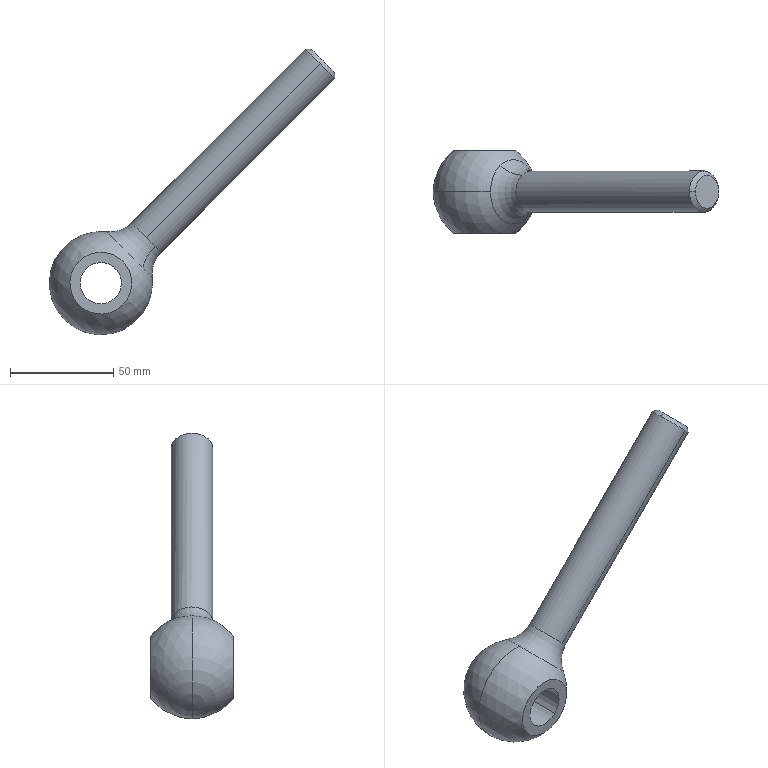Part | 1 solid | 13 faces | box 138.299 x 40 x 138.299 mm | volume 90064 mm3 | cylinder 4 | plane 3 | cone 2 | torus 2 | sphere 2 | commonest cylinder face diameters 20 x4
STEP:
#1=CARTESIAN_POINT('',(0.,0.,0.));
#2=DIRECTION('',(0.,0.,1.));
#3=DIRECTION('',(1.,0.,0.));
#4=AXIS2_PLACEMENT_3D('',#1,#2,#3);
#5=CARTESIAN_POINT('',(97.888,511.5,-299.372));
#6=VERTEX_POINT('',#5);
#7=CARTESIAN_POINT('',(13.739,511.5,-383.521));
#8=VERTEX_POINT('',#7);
#9=CARTESIAN_POINT('',(97.888,511.5,-299.372));
#10=DIRECTION('',(-0.7071,0.,-0.7071));
#11=VECTOR('',#10,1.);
#12=LINE('',#9,#11);
#13=CARTESIAN_POINT('',(-68.056,501.5,-465.316));
#14=DIRECTION('',(-0.7071,0.,-0.7071));
#15=DIRECTION('',(-0.7071,0.,0.7071));
#16=AXIS2_PLACEMENT_3D('',#13,#14,#15);
#17=CYLINDRICAL_SURFACE('',#16,10.);
#18=CARTESIAN_POINT('',(1.571,-234.68));
#19=DIRECTION('',(0.,1.));
#20=VECTOR('',#19,1.);
#21=LINE('',#18,#20);
#22=(GEOMETRIC_REPRESENTATION_CONTEXT(2)PARAMETRIC_REPRESENTATION_CONTEXT()REPRESENTATION_CONTEXT('',''));
#23=DEFINITIONAL_REPRESENTATION('',(#21),#22);
#24=PCURVE('',#17,#23);
#25=CARTESIAN_POINT('',(-68.056,501.5,-465.316));
#26=DIRECTION('',(-0.7071,0.,-0.7071));
#27=DIRECTION('',(0.7071,0.,-0.7071));
#28=AXIS2_PLACEMENT_3D('',#25,#26,#27);
#29=CYLINDRICAL_SURFACE('',#28,10.);
#30=CARTESIAN_POINT('',(4.712,-234.68));
#31=DIRECTION('',(0.,1.));
#32=VECTOR('',#31,1.);
#33=LINE('',#30,#32);
#34=(GEOMETRIC_REPRESENTATION_CONTEXT(2)PARAMETRIC_REPRESENTATION_CONTEXT()REPRESENTATION_CONTEXT('',''));
#35=DEFINITIONAL_REPRESENTATION('',(#33),#34);
#36=PCURVE('',#29,#35);
#37=SURFACE_CURVE('',#12,(#24,#36),.PCURVE_S1.);
#38=EDGE_CURVE('',#6,#8,#37,.T.);
#39=ORIENTED_EDGE('',*,*,#38,.F.);
#40=CARTESIAN_POINT('',(104.959,501.5,-306.443));
#41=VERTEX_POINT('',#40);
#42=CARTESIAN_POINT('',(97.888,501.5,-299.372));
#43=DIRECTION('',(-0.7071,0.,-0.7071));
#44=DIRECTION('',(0.7071,0.,-0.7071));
#45=AXIS2_PLACEMENT_3D('',#42,#43,#44);
#46=CIRCLE('',#45,10.);
#47=CARTESIAN_POINT('',(-3.142,-234.68));
#48=DIRECTION('',(1.,0.));
#49=VECTOR('',#48,1.);
#50=LINE('',#47,#49);
#51=(GEOMETRIC_REPRESENTATION_CONTEXT(2)PARAMETRIC_REPRESENTATION_CONTEXT()REPRESENTATION_CONTEXT('',''));
#52=DEFINITIONAL_REPRESENTATION('',(#50),#51);
#53=PCURVE('',#17,#52);
#54=CARTESIAN_POINT('',(97.888,501.5,-299.372));
#55=DIRECTION('',(-0.7071,0.,-0.7071));
#56=DIRECTION('',(0.,-1.,0.));
#57=AXIS2_PLACEMENT_3D('',#54,#55,#56);
#58=CONICAL_SURFACE('',#57,10.,0.7854);
#59=CARTESIAN_POINT('',(-1.571,0.));
#60=DIRECTION('',(1.,0.));
#61=VECTOR('',#60,1.);
#62=LINE('',#59,#61);
#63=(GEOMETRIC_REPRESENTATION_CONTEXT(2)PARAMETRIC_REPRESENTATION_CONTEXT()REPRESENTATION_CONTEXT('',''));
#64=DEFINITIONAL_REPRESENTATION('',(#62),#63);
#65=PCURVE('',#58,#64);
#66=SURFACE_CURVE('',#46,(#53,#65),.PCURVE_S1.);
#67=EDGE_CURVE('',#6,#41,#66,.T.);
#68=ORIENTED_EDGE('',*,*,#67,.T.);
#69=CARTESIAN_POINT('',(97.888,491.5,-299.372));
#70=VERTEX_POINT('',#69);
#71=CARTESIAN_POINT('',(97.888,501.5,-299.372));
#72=DIRECTION('',(-0.7071,0.,-0.7071));
#73=DIRECTION('',(0.7071,0.,-0.7071));
#74=AXIS2_PLACEMENT_3D('',#71,#72,#73);
#75=CIRCLE('',#74,10.);
#76=CARTESIAN_POINT('',(3.142,-234.68));
#77=DIRECTION('',(1.,0.));
#78=VECTOR('',#77,1.);
#79=LINE('',#76,#78);
#80=(GEOMETRIC_REPRESENTATION_CONTEXT(2)PARAMETRIC_REPRESENTATION_CONTEXT()REPRESENTATION_CONTEXT('',''));
#81=DEFINITIONAL_REPRESENTATION('',(#79),#80);
#82=PCURVE('',#17,#81);
#83=CARTESIAN_POINT('',(97.888,501.5,-299.372));
#84=DIRECTION('',(-0.7071,0.,-0.7071));
#85=DIRECTION('',(0.,1.,0.));
#86=AXIS2_PLACEMENT_3D('',#83,#84,#85);
#87=CONICAL_SURFACE('',#86,10.,0.7854);
#88=CARTESIAN_POINT('',(1.571,0.));
#89=DIRECTION('',(1.,0.));
#90=VECTOR('',#89,1.);
#91=LINE('',#88,#90);
#92=(GEOMETRIC_REPRESENTATION_CONTEXT(2)PARAMETRIC_REPRESENTATION_CONTEXT()REPRESENTATION_CONTEXT('',''));
#93=DEFINITIONAL_REPRESENTATION('',(#91),#92);
#94=PCURVE('',#87,#93);
#95=SURFACE_CURVE('',#75,(#82,#94),.PCURVE_S1.);
#96=EDGE_CURVE('',#41,#70,#95,.T.);
#97=ORIENTED_EDGE('',*,*,#96,.T.);
#98=CARTESIAN_POINT('',(13.739,491.5,-383.521));
#99=VERTEX_POINT('',#98);
#100=CARTESIAN_POINT('',(97.888,491.5,-299.372));
#101=DIRECTION('',(-0.7071,0.,-0.7071));
#102=VECTOR('',#101,1.);
#103=LINE('',#100,#102);
#104=CARTESIAN_POINT('',(4.712,-234.68));
#105=DIRECTION('',(0.,1.));
#106=VECTOR('',#105,1.);
#107=LINE('',#104,#106);
#108=(GEOMETRIC_REPRESENTATION_CONTEXT(2)PARAMETRIC_REPRESENTATION_CONTEXT()REPRESENTATION_CONTEXT('',''));
#109=DEFINITIONAL_REPRESENTATION('',(#107),#108);
#110=PCURVE('',#17,#109);
#111=CARTESIAN_POINT('',(1.571,-234.68));
#112=DIRECTION('',(0.,1.));
#113=VECTOR('',#112,1.);
#114=LINE('',#111,#113);
#115=(GEOMETRIC_REPRESENTATION_CONTEXT(2)PARAMETRIC_REPRESENTATION_CONTEXT()REPRESENTATION_CONTEXT('',''));
#116=DEFINITIONAL_REPRESENTATION('',(#114),#115);
#117=PCURVE('',#29,#116);
#118=SURFACE_CURVE('',#103,(#110,#117),.PCURVE_S1.);
#119=EDGE_CURVE('',#70,#99,#118,.T.);
#120=ORIENTED_EDGE('',*,*,#119,.T.);
#121=CARTESIAN_POINT('',(17.896,493.41,-387.677));
#122=VERTEX_POINT('',#121);
#123=CARTESIAN_POINT('',(13.739,501.5,-383.521));
#124=DIRECTION('',(-0.7071,0.,-0.7071));
#125=DIRECTION('',(0.,-1.,0.));
#126=AXIS2_PLACEMENT_3D('',#123,#124,#125);
#127=CIRCLE('',#126,10.);
#128=CARTESIAN_POINT('',(-1.571,-115.676));
#129=DIRECTION('',(1.,0.));
#130=VECTOR('',#129,1.);
#131=LINE('',#128,#130);
#132=(GEOMETRIC_REPRESENTATION_CONTEXT(2)PARAMETRIC_REPRESENTATION_CONTEXT()REPRESENTATION_CONTEXT('',''));
#133=DEFINITIONAL_REPRESENTATION('',(#131),#132);
#134=PCURVE('',#17,#133);
#135=CARTESIAN_POINT('',(13.739,501.5,-383.521));
#136=DIRECTION('',(-0.7071,0.,-0.7071));
#137=DIRECTION('',(0.5721,0.5878,-0.5721));
#138=AXIS2_PLACEMENT_3D('',#135,#136,#137);
#139=TOROIDAL_SURFACE('',#138,25.,15.);
#140=CARTESIAN_POINT('',(-4.084,3.142));
#141=DIRECTION('',(1.,0.));
#142=VECTOR('',#141,1.);
#143=LINE('',#140,#142);
#144=(GEOMETRIC_REPRESENTATION_CONTEXT(2)PARAMETRIC_REPRESENTATION_CONTEXT()REPRESENTATION_CONTEXT('',''));
#145=DEFINITIONAL_REPRESENTATION('',(#143),#144);
#146=PCURVE('',#139,#145);
#147=SURFACE_CURVE('',#127,(#134,#146),.PCURVE_S1.);
#148=EDGE_CURVE('',#122,#99,#147,.T.);
#149=ORIENTED_EDGE('',*,*,#148,.F.);
#150=CARTESIAN_POINT('',(13.739,501.5,-383.521));
#151=DIRECTION('',(-0.7071,0.,-0.7071));
#152=DIRECTION('',(0.,-1.,0.));
#153=AXIS2_PLACEMENT_3D('',#150,#151,#152);
#154=CIRCLE('',#153,10.);
#155=CARTESIAN_POINT('',(-1.571,-115.676));
#156=DIRECTION('',(1.,0.));
#157=VECTOR('',#156,1.);
#158=LINE('',#155,#157);
#159=(GEOMETRIC_REPRESENTATION_CONTEXT(2)PARAMETRIC_REPRESENTATION_CONTEXT()REPRESENTATION_CONTEXT('',''));
#160=DEFINITIONAL_REPRESENTATION('',(#158),#159);
#161=PCURVE('',#17,#160);
#162=CARTESIAN_POINT('',(13.739,501.5,-383.521));
#163=DIRECTION('',(-0.7071,0.,-0.7071));
#164=DIRECTION('',(-0.5721,-0.5878,0.5721));
#165=AXIS2_PLACEMENT_3D('',#162,#163,#164);
#166=TOROIDAL_SURFACE('',#165,25.,15.);
#167=CARTESIAN_POINT('',(-0.9425,3.142));
#168=DIRECTION('',(1.,0.));
#169=VECTOR('',#168,1.);
#170=LINE('',#167,#169);
#171=(GEOMETRIC_REPRESENTATION_CONTEXT(2)PARAMETRIC_REPRESENTATION_CONTEXT()REPRESENTATION_CONTEXT('',''));
#172=DEFINITIONAL_REPRESENTATION('',(#170),#171);
#173=PCURVE('',#166,#172);
#174=SURFACE_CURVE('',#154,(#161,#173),.PCURVE_S1.);
#175=EDGE_CURVE('',#8,#122,#174,.T.);
#176=ORIENTED_EDGE('',*,*,#175,.F.);
#177=EDGE_LOOP('',(#39,#68,#97,#120,#149,#176));
#178=FACE_BOUND('',#177,.T.);
#179=ADVANCED_FACE('',(#178),#17,.T.);
#180=CARTESIAN_POINT('',(93.646,501.5,-292.301));
#181=VERTEX_POINT('',#180);
#182=CARTESIAN_POINT('',(90.817,501.5,-292.301));
#183=VERTEX_POINT('',#182);
#184=CARTESIAN_POINT('',(93.646,501.5,-292.301));
#185=DIRECTION('',(-1.,0.,-0.000000001));
#186=VECTOR('',#185,1.);
#187=LINE('',#184,#186);
#188=CARTESIAN_POINT('',(1.571,-2.));
#189=DIRECTION('',(0.,1.));
#190=VECTOR('',#189,1.);
#191=LINE('',#188,#190);
#192=(GEOMETRIC_REPRESENTATION_CONTEXT(2)PARAMETRIC_REPRESENTATION_CONTEXT()REPRESENTATION_CONTEXT('',''));
#193=DEFINITIONAL_REPRESENTATION('',(#191),#192);
#194=PCURVE('',#58,#193);
#195=CARTESIAN_POINT('',(4.712,-2.));
#196=DIRECTION('',(0.,1.));
#197=VECTOR('',#196,1.);
#198=LINE('',#195,#197);
#199=(GEOMETRIC_REPRESENTATION_CONTEXT(2)PARAMETRIC_REPRESENTATION_CONTEXT()REPRESENTATION_CONTEXT('',''));
#200=DEFINITIONAL_REPRESENTATION('',(#198),#199);
#201=PCURVE('',#87,#200);
#202=SURFACE_CURVE('',#187,(#194,#201),.PCURVE_S1.);
#203=EDGE_CURVE('',#181,#183,#202,.T.);
#204=ORIENTED_EDGE('',*,*,#203,.F.);
#205=CARTESIAN_POINT('',(104.959,501.5,-303.614));
#206=VERTEX_POINT('',#205);
#207=CARTESIAN_POINT('',(99.303,501.5,-297.958));
#208=DIRECTION('',(0.7071,0.,0.7071));
#209=DIRECTION('',(0.7071,0.,-0.7071));
#210=AXIS2_PLACEMENT_3D('',#207,#208,#209);
#211=CIRCLE('',#210,8.);
#212=CARTESIAN_POINT('',(4.712,-2.));
#213=DIRECTION('',(-1.,0.));
#214=VECTOR('',#213,1.);
#215=LINE('',#212,#214);
#216=(GEOMETRIC_REPRESENTATION_CONTEXT(2)PARAMETRIC_REPRESENTATION_CONTEXT()REPRESENTATION_CONTEXT('',''));
#217=DEFINITIONAL_REPRESENTATION('',(#215),#216);
#218=PCURVE('',#58,#217);
#219=CARTESIAN_POINT('',(93.646,501.5,-292.301));
#220=DIRECTION('',(0.7071,0.,0.7071));
#221=DIRECTION('',(0.,1.,0.));
#222=AXIS2_PLACEMENT_3D('',#219,#220,#221);
#223=PLANE('',#222);
#224=CARTESIAN_POINT('',(0.,-8.));
#225=DIRECTION('',(0.,-1.));
#226=AXIS2_PLACEMENT_2D('',#224,#225);
#227=CIRCLE('',#226,8.);
#228=(GEOMETRIC_REPRESENTATION_CONTEXT(2)PARAMETRIC_REPRESENTATION_CONTEXT()REPRESENTATION_CONTEXT('',''));
#229=DEFINITIONAL_REPRESENTATION('',(#227),#228);
#230=PCURVE('',#223,#229);
#231=SURFACE_CURVE('',#211,(#218,#230),.PCURVE_S1.);
#232=EDGE_CURVE('',#206,#181,#231,.T.);
#233=ORIENTED_EDGE('',*,*,#232,.F.);
#234=CARTESIAN_POINT('',(104.959,501.5,-303.614));
#235=DIRECTION('',(0.,0.,-1.));
#236=VECTOR('',#235,1.);
#237=LINE('',#234,#236);
#238=CARTESIAN_POINT('',(4.712,-2.));
#239=DIRECTION('',(0.,1.));
#240=VECTOR('',#239,1.);
#241=LINE('',#238,#240);
#242=(GEOMETRIC_REPRESENTATION_CONTEXT(2)PARAMETRIC_REPRESENTATION_CONTEXT()REPRESENTATION_CONTEXT('',''));
#243=DEFINITIONAL_REPRESENTATION('',(#241),#242);
#244=PCURVE('',#58,#243);
#245=CARTESIAN_POINT('',(1.571,-2.));
#246=DIRECTION('',(0.,1.));
#247=VECTOR('',#246,1.);
#248=LINE('',#245,#247);
#249=(GEOMETRIC_REPRESENTATION_CONTEXT(2)PARAMETRIC_REPRESENTATION_CONTEXT()REPRESENTATION_CONTEXT('',''));
#250=DEFINITIONAL_REPRESENTATION('',(#248),#249);
#251=PCURVE('',#87,#250);
#252=SURFACE_CURVE('',#237,(#244,#251),.PCURVE_S1.);
#253=EDGE_CURVE('',#206,#41,#252,.T.);
#254=ORIENTED_EDGE('',*,*,#253,.T.);
#255=ORIENTED_EDGE('',*,*,#67,.F.);
#256=CARTESIAN_POINT('',(97.888,501.5,-299.372));
#257=DIRECTION('',(-0.7071,0.,-0.7071));
#258=DIRECTION('',(0.7071,0.,-0.7071));
#259=AXIS2_PLACEMENT_3D('',#256,#257,#258);
#260=CIRCLE('',#259,10.);
#261=CARTESIAN_POINT('',(-1.571,0.));
#262=DIRECTION('',(1.,0.));
#263=VECTOR('',#262,1.);
#264=LINE('',#261,#263);
#265=(GEOMETRIC_REPRESENTATION_CONTEXT(2)PARAMETRIC_REPRESENTATION_CONTEXT()REPRESENTATION_CONTEXT('',''));
#266=DEFINITIONAL_REPRESENTATION('',(#264),#265);
#267=PCURVE('',#58,#266);
#268=CARTESIAN_POINT('',(0.,-234.68));
#269=DIRECTION('',(1.,0.));
#270=VECTOR('',#269,1.);
#271=LINE('',#268,#270);
#272=(GEOMETRIC_REPRESENTATION_CONTEXT(2)PARAMETRIC_REPRESENTATION_CONTEXT()REPRESENTATION_CONTEXT('',''));
#273=DEFINITIONAL_REPRESENTATION('',(#271),#272);
#274=PCURVE('',#29,#273);
#275=SURFACE_CURVE('',#260,(#267,#274),.PCURVE_S1.);
#276=EDGE_CURVE('',#183,#6,#275,.T.);
#277=ORIENTED_EDGE('',*,*,#276,.F.);
#278=EDGE_LOOP('',(#204,#233,#254,#255,#277));
#279=FACE_BOUND('',#278,.T.);
#280=ADVANCED_FACE('',(#279),#58,.T.);
#281=ORIENTED_EDGE('',*,*,#232,.T.);
#282=CARTESIAN_POINT('',(99.303,501.5,-297.958));
#283=DIRECTION('',(0.7071,0.,0.7071));
#284=DIRECTION('',(0.7071,0.,-0.7071));
#285=AXIS2_PLACEMENT_3D('',#282,#283,#284);
#286=CIRCLE('',#285,8.);
#287=CARTESIAN_POINT('',(0.,-8.));
#288=DIRECTION('',(0.,-1.));
#289=AXIS2_PLACEMENT_2D('',#287,#288);
#290=CIRCLE('',#289,8.);
#291=(GEOMETRIC_REPRESENTATION_CONTEXT(2)PARAMETRIC_REPRESENTATION_CONTEXT()REPRESENTATION_CONTEXT('',''));
#292=DEFINITIONAL_REPRESENTATION('',(#290),#291);
#293=PCURVE('',#223,#292);
#294=CARTESIAN_POINT('',(7.854,-2.));
#295=DIRECTION('',(-1.,0.));
#296=VECTOR('',#295,1.);
#297=LINE('',#294,#296);
#298=(GEOMETRIC_REPRESENTATION_CONTEXT(2)PARAMETRIC_REPRESENTATION_CONTEXT()REPRESENTATION_CONTEXT('',''));
#299=DEFINITIONAL_REPRESENTATION('',(#297),#298);
#300=PCURVE('',#87,#299);
#301=SURFACE_CURVE('',#286,(#293,#300),.PCURVE_S1.);
#302=EDGE_CURVE('',#181,#206,#301,.T.);
#303=ORIENTED_EDGE('',*,*,#302,.T.);
#304=EDGE_LOOP('',(#281,#303));
#305=FACE_BOUND('',#304,.T.);
#306=ADVANCED_FACE('',(#305),#223,.T.);
#307=CARTESIAN_POINT('',(-1.034,514.141,-385.306));
#308=VERTEX_POINT('',#307);
#309=CARTESIAN_POINT('',(16.508,501.5,-402.849));
#310=VERTEX_POINT('',#309);
#311=CARTESIAN_POINT('',(5.46,501.5,-391.8));
#312=DIRECTION('',(-0.7071,0.,-0.7071));
#313=DIRECTION('',(0.7071,0.,-0.7071));
#314=AXIS2_PLACEMENT_3D('',#311,#312,#313);
#315=CIRCLE('',#314,15.625);
#316=CARTESIAN_POINT('',(-2.513,2.246));
#317=DIRECTION('',(1.,0.));
#318=VECTOR('',#317,1.);
#319=LINE('',#316,#318);
#320=(GEOMETRIC_REPRESENTATION_CONTEXT(2)PARAMETRIC_REPRESENTATION_CONTEXT()REPRESENTATION_CONTEXT('',''));
#321=DEFINITIONAL_REPRESENTATION('',(#319),#320);
#322=PCURVE('',#166,#321);
#323=CARTESIAN_POINT('',(-8.34,501.5,-405.6));
#324=DIRECTION('',(-0.7071,0.,-0.7071));
#325=DIRECTION('',(0.,-1.,0.));
#326=AXIS2_PLACEMENT_3D('',#323,#324,#325);
#327=SPHERICAL_SURFACE('',#326,25.);
#328=CARTESIAN_POINT('',(-1.571,-0.8957));
#329=DIRECTION('',(1.,0.));
#330=VECTOR('',#329,1.);
#331=LINE('',#328,#330);
#332=(GEOMETRIC_REPRESENTATION_CONTEXT(2)PARAMETRIC_REPRESENTATION_CONTEXT()REPRESENTATION_CONTEXT('',''));
#333=DEFINITIONAL_REPRESENTATION('',(#331),#332);
#334=PCURVE('',#327,#333);
#335=SURFACE_CURVE('',#315,(#322,#334),.PCURVE_S1.);
#336=EDGE_CURVE('',#308,#310,#335,.T.);
#337=ORIENTED_EDGE('',*,*,#336,.T.);
#338=CARTESIAN_POINT('',(11.954,488.859,-398.295));
#339=VERTEX_POINT('',#338);
#340=CARTESIAN_POINT('',(5.46,501.5,-391.8));
#341=DIRECTION('',(-0.7071,0.,-0.7071));
#342=DIRECTION('',(0.7071,0.,-0.7071));
#343=AXIS2_PLACEMENT_3D('',#340,#341,#342);
#344=CIRCLE('',#343,15.625);
#345=CARTESIAN_POINT('',(3.77,2.246));
#346=DIRECTION('',(1.,0.));
#347=VECTOR('',#346,1.);
#348=LINE('',#345,#347);
#349=(GEOMETRIC_REPRESENTATION_CONTEXT(2)PARAMETRIC_REPRESENTATION_CONTEXT()REPRESENTATION_CONTEXT('',''));
#350=DEFINITIONAL_REPRESENTATION('',(#348),#349);
#351=PCURVE('',#166,#350);
#352=CARTESIAN_POINT('',(-8.34,501.5,-405.6));
#353=DIRECTION('',(-0.7071,0.,-0.7071));
#354=DIRECTION('',(0.,1.,0.));
#355=AXIS2_PLACEMENT_3D('',#352,#353,#354);
#356=SPHERICAL_SURFACE('',#355,25.);
#357=CARTESIAN_POINT('',(1.571,-0.8957));
#358=DIRECTION('',(1.,0.));
#359=VECTOR('',#358,1.);
#360=LINE('',#357,#359);
#361=(GEOMETRIC_REPRESENTATION_CONTEXT(2)PARAMETRIC_REPRESENTATION_CONTEXT()REPRESENTATION_CONTEXT('',''));
#362=DEFINITIONAL_REPRESENTATION('',(#360),#361);
#363=PCURVE('',#356,#362);
#364=SURFACE_CURVE('',#344,(#351,#363),.PCURVE_S1.);
#365=EDGE_CURVE('',#310,#339,#364,.T.);
#366=ORIENTED_EDGE('',*,*,#365,.T.);
#367=CARTESIAN_POINT('',(24.13,481.275,-393.911));
#368=DIRECTION('',(-0.5721,-0.5878,0.5721));
#369=DIRECTION('',(-0.4156,0.809,0.4156));
#370=AXIS2_PLACEMENT_3D('',#367,#368,#369);
#371=CIRCLE('',#370,15.);
#372=CARTESIAN_POINT('',(4.712,3.142));
#373=DIRECTION('',(0.,-1.));
#374=VECTOR('',#373,1.);
#375=LINE('',#372,#374);
#376=(GEOMETRIC_REPRESENTATION_CONTEXT(2)PARAMETRIC_REPRESENTATION_CONTEXT()REPRESENTATION_CONTEXT('',''));
#377=DEFINITIONAL_REPRESENTATION('',(#375),#376);
#378=PCURVE('',#166,#377);
#379=CARTESIAN_POINT('',(1.571,3.142));
#380=DIRECTION('',(0.,-1.));
#381=VECTOR('',#380,1.);
#382=LINE('',#379,#381);
#383=(GEOMETRIC_REPRESENTATION_CONTEXT(2)PARAMETRIC_REPRESENTATION_CONTEXT()REPRESENTATION_CONTEXT('',''));
#384=DEFINITIONAL_REPRESENTATION('',(#382),#383);
#385=PCURVE('',#139,#384);
#386=SURFACE_CURVE('',#371,(#378,#385),.PCURVE_S1.);
#387=EDGE_CURVE('',#122,#339,#386,.T.);
#388=ORIENTED_EDGE('',*,*,#387,.F.);
#389=ORIENTED_EDGE('',*,*,#175,.F.);
#390=CARTESIAN_POINT('',(9.583,509.59,-379.364));
#391=VERTEX_POINT('',#390);
#392=CARTESIAN_POINT('',(13.739,501.5,-383.521));
#393=DIRECTION('',(-0.7071,0.,-0.7071));
#394=DIRECTION('',(0.,-1.,0.));
#395=AXIS2_PLACEMENT_3D('',#392,#393,#394);
#396=CIRCLE('',#395,10.);
#397=CARTESIAN_POINT('',(-0.9425,3.142));
#398=DIRECTION('',(1.,0.));
#399=VECTOR('',#398,1.);
#400=LINE('',#397,#399);
#401=(GEOMETRIC_REPRESENTATION_CONTEXT(2)PARAMETRIC_REPRESENTATION_CONTEXT()REPRESENTATION_CONTEXT('',''));
#402=DEFINITIONAL_REPRESENTATION('',(#400),#401);
#403=PCURVE('',#166,#402);
#404=CARTESIAN_POINT('',(1.571,-115.676));
#405=DIRECTION('',(1.,0.));
#406=VECTOR('',#405,1.);
#407=LINE('',#404,#406);
#408=(GEOMETRIC_REPRESENTATION_CONTEXT(2)PARAMETRIC_REPRESENTATION_CONTEXT()REPRESENTATION_CONTEXT('',''));
#409=DEFINITIONAL_REPRESENTATION('',(#407),#408);
#410=PCURVE('',#29,#409);
#411=SURFACE_CURVE('',#396,(#403,#410),.PCURVE_S1.);
#412=EDGE_CURVE('',#391,#8,#411,.T.);
#413=ORIENTED_EDGE('',*,*,#412,.F.);
#414=CARTESIAN_POINT('',(3.349,521.725,-373.13));
#415=DIRECTION('',(0.5721,0.5878,-0.5721));
#416=DIRECTION('',(0.4156,-0.809,-0.4156));
#417=AXIS2_PLACEMENT_3D('',#414,#415,#416);
#418=CIRCLE('',#417,15.);
#419=CARTESIAN_POINT('',(1.571,3.142));
#420=DIRECTION('',(0.,-1.));
#421=VECTOR('',#420,1.);
#422=LINE('',#419,#421);
#423=(GEOMETRIC_REPRESENTATION_CONTEXT(2)PARAMETRIC_REPRESENTATION_CONTEXT()REPRESENTATION_CONTEXT('',''));
#424=DEFINITIONAL_REPRESENTATION('',(#422),#423);
#425=PCURVE('',#166,#424);
#426=CARTESIAN_POINT('',(4.712,3.142));
#427=DIRECTION('',(0.,-1.));
#428=VECTOR('',#427,1.);
#429=LINE('',#426,#428);
#430=(GEOMETRIC_REPRESENTATION_CONTEXT(2)PARAMETRIC_REPRESENTATION_CONTEXT()REPRESENTATION_CONTEXT('',''));
#431=DEFINITIONAL_REPRESENTATION('',(#429),#430);
#432=PCURVE('',#139,#431);
#433=SURFACE_CURVE('',#418,(#425,#432),.PCURVE_S1.);
#434=EDGE_CURVE('',#391,#308,#433,.T.);
#435=ORIENTED_EDGE('',*,*,#434,.T.);
#436=EDGE_LOOP('',(#337,#366,#388,#389,#413,#435));
#437=FACE_BOUND('',#436,.F.);
#438=ADVANCED_FACE('',(#437),#166,.F.);
#439=CARTESIAN_POINT('',(-26.018,501.5,-423.278));
#440=VERTEX_POINT('',#439);
#441=CARTESIAN_POINT('',(-5.589,501.5,-380.752));
#442=VERTEX_POINT('',#441);
#443=CARTESIAN_POINT('',(-8.34,501.5,-405.6));
#444=DIRECTION('',(0.,1.,0.));
#445=DIRECTION('',(-0.7071,0.,-0.7071));
#446=AXIS2_PLACEMENT_3D('',#443,#444,#445);
#447=CIRCLE('',#446,25.);
#448=CARTESIAN_POINT('',(1.571,1.571));
#449=CARTESIAN_POINT('',(1.571,1.533));
#450=CARTESIAN_POINT('',(1.571,1.459));
#451=CARTESIAN_POINT('',(1.571,1.347));
#452=CARTESIAN_POINT('',(1.571,1.234));
#453=CARTESIAN_POINT('',(1.571,1.122));
#454=CARTESIAN_POINT('',(1.571,1.01));
#455=CARTESIAN_POINT('',(1.571,0.8981));
#456=CARTESIAN_POINT('',(1.571,0.786));
#457=CARTESIAN_POINT('',(1.571,0.6739));
#458=CARTESIAN_POINT('',(1.571,0.5618));
#459=CARTESIAN_POINT('',(1.571,0.4497));
#460=CARTESIAN_POINT('',(1.571,0.3376));
#461=CARTESIAN_POINT('',(1.571,0.2255));
#462=CARTESIAN_POINT('',(1.571,0.1133));
#463=CARTESIAN_POINT('',(1.571,0.00123));
#464=CARTESIAN_POINT('',(1.571,-0.1109));
#465=CARTESIAN_POINT('',(1.571,-0.223));
#466=CARTESIAN_POINT('',(1.571,-0.3351));
#467=CARTESIAN_POINT('',(1.571,-0.4472));
#468=CARTESIAN_POINT('',(1.571,-0.5593));
#469=CARTESIAN_POINT('',(1.571,-0.6714));
#470=CARTESIAN_POINT('',(1.571,-0.7836));
#471=CARTESIAN_POINT('',(1.571,-0.8583));
#472=CARTESIAN_POINT('',(1.571,-0.8957));
#473=B_SPLINE_CURVE_WITH_KNOTS('',3,(#448,#449,#450,#451,#452,#453,#454,#455,#456,#457,#458,#459,#460,#461,#462,#463,#464,#465,#466,#467,#468,#469,#470,#471,#472),.UNSPECIFIED.,.F.,.F.,(4,1,1,1,1,1,1,1,1,1,1,1,1,1,1,1,1,1,1,1,1,1,4),(0.,0.1121,0.2242,0.3363,0.4484,0.5606,0.6727,0.7848,0.8969,1.009,1.121,1.233,1.345,1.457,1.57,1.682,1.794,1.906,2.018,2.13,2.242,2.354,2.466),.QUASI_UNIFORM_KNOTS.);
#474=(GEOMETRIC_REPRESENTATION_CONTEXT(2)PARAMETRIC_REPRESENTATION_CONTEXT()REPRESENTATION_CONTEXT('',''));
#475=DEFINITIONAL_REPRESENTATION('',(#473),#474);
#476=PCURVE('',#327,#475);
#477=CARTESIAN_POINT('',(4.712,1.571));
#478=CARTESIAN_POINT('',(4.712,1.533));
#479=CARTESIAN_POINT('',(4.712,1.459));
#480=CARTESIAN_POINT('',(4.712,1.347));
#481=CARTESIAN_POINT('',(4.712,1.234));
#482=CARTESIAN_POINT('',(4.712,1.122));
#483=CARTESIAN_POINT('',(4.712,1.01));
#484=CARTESIAN_POINT('',(4.712,0.8981));
#485=CARTESIAN_POINT('',(4.712,0.786));
#486=CARTESIAN_POINT('',(4.712,0.6739));
#487=CARTESIAN_POINT('',(4.712,0.5618));
#488=CARTESIAN_POINT('',(4.712,0.4497));
#489=CARTESIAN_POINT('',(4.712,0.3376));
#490=CARTESIAN_POINT('',(4.712,0.2255));
#491=CARTESIAN_POINT('',(4.712,0.1133));
#492=CARTESIAN_POINT('',(4.712,0.00123));
#493=CARTESIAN_POINT('',(4.712,-0.1109));
#494=CARTESIAN_POINT('',(4.712,-0.223));
#495=CARTESIAN_POINT('',(4.712,-0.3351));
#496=CARTESIAN_POINT('',(4.712,-0.4472));
#497=CARTESIAN_POINT('',(4.712,-0.5593));
#498=CARTESIAN_POINT('',(4.712,-0.6714));
#499=CARTESIAN_POINT('',(4.712,-0.7836));
#500=CARTESIAN_POINT('',(4.712,-0.8583));
#501=CARTESIAN_POINT('',(4.712,-0.8957));
#502=B_SPLINE_CURVE_WITH_KNOTS('',3,(#477,#478,#479,#480,#481,#482,#483,#484,#485,#486,#487,#488,#489,#490,#491,#492,#493,#494,#495,#496,#497,#498,#499,#500,#501),.UNSPECIFIED.,.F.,.F.,(4,1,1,1,1,1,1,1,1,1,1,1,1,1,1,1,1,1,1,1,1,1,4),(0.,0.1121,0.2242,0.3363,0.4484,0.5606,0.6727,0.7848,0.8969,1.009,1.121,1.233,1.345,1.457,1.57,1.682,1.794,1.906,2.018,2.13,2.242,2.354,2.466),.QUASI_UNIFORM_KNOTS.);
#503=(GEOMETRIC_REPRESENTATION_CONTEXT(2)PARAMETRIC_REPRESENTATION_CONTEXT()REPRESENTATION_CONTEXT('',''));
#504=DEFINITIONAL_REPRESENTATION('',(#502),#503);
#505=PCURVE('',#356,#504);
#506=SURFACE_CURVE('',#447,(#476,#505),.PCURVE_S1.);
#507=EDGE_CURVE('',#440,#442,#506,.T.);
#508=ORIENTED_EDGE('',*,*,#507,.T.);
#509=CARTESIAN_POINT('',(5.46,501.5,-391.8));
#510=DIRECTION('',(-0.7071,0.,-0.7071));
#511=DIRECTION('',(0.7071,0.,-0.7071));
#512=AXIS2_PLACEMENT_3D('',#509,#510,#511);
#513=CIRCLE('',#512,15.625);
#514=CARTESIAN_POINT('',(-1.571,-0.8957));
#515=DIRECTION('',(1.,0.));
#516=VECTOR('',#515,1.);
#517=LINE('',#514,#516);
#518=(GEOMETRIC_REPRESENTATION_CONTEXT(2)PARAMETRIC_REPRESENTATION_CONTEXT()REPRESENTATION_CONTEXT('',''));
#519=DEFINITIONAL_REPRESENTATION('',(#517),#518);
#520=PCURVE('',#327,#519);
#521=CARTESIAN_POINT('',(0.6283,2.246));
#522=DIRECTION('',(1.,0.));
#523=VECTOR('',#522,1.);
#524=LINE('',#521,#523);
#525=(GEOMETRIC_REPRESENTATION_CONTEXT(2)PARAMETRIC_REPRESENTATION_CONTEXT()REPRESENTATION_CONTEXT('',''));
#526=DEFINITIONAL_REPRESENTATION('',(#524),#525);
#527=PCURVE('',#139,#526);
#528=SURFACE_CURVE('',#513,(#520,#527),.PCURVE_S1.);
#529=EDGE_CURVE('',#442,#308,#528,.T.);
#530=ORIENTED_EDGE('',*,*,#529,.T.);
#531=ORIENTED_EDGE('',*,*,#336,.T.);
#532=CARTESIAN_POINT('',(-8.34,501.5,-405.6));
#533=DIRECTION('',(0.,-1.,0.));
#534=DIRECTION('',(-0.7071,0.,-0.7071));
#535=AXIS2_PLACEMENT_3D('',#532,#533,#534);
#536=CIRCLE('',#535,25.);
#537=CARTESIAN_POINT('',(4.712,1.571));
#538=DIRECTION('',(0.,-1.));
#539=VECTOR('',#538,1.);
#540=LINE('',#537,#539);
#541=(GEOMETRIC_REPRESENTATION_CONTEXT(2)PARAMETRIC_REPRESENTATION_CONTEXT()REPRESENTATION_CONTEXT('',''));
#542=DEFINITIONAL_REPRESENTATION('',(#540),#541);
#543=PCURVE('',#327,#542);
#544=CARTESIAN_POINT('',(1.571,1.571));
#545=DIRECTION('',(0.,-1.));
#546=VECTOR('',#545,1.);
#547=LINE('',#544,#546);
#548=(GEOMETRIC_REPRESENTATION_CONTEXT(2)PARAMETRIC_REPRESENTATION_CONTEXT()REPRESENTATION_CONTEXT('',''));
#549=DEFINITIONAL_REPRESENTATION('',(#547),#548);
#550=PCURVE('',#356,#549);
#551=SURFACE_CURVE('',#536,(#543,#550),.PCURVE_S1.);
#552=EDGE_CURVE('',#440,#310,#551,.T.);
#553=ORIENTED_EDGE('',*,*,#552,.F.);
#554=EDGE_LOOP('',(#508,#530,#531,#553));
#555=FACE_BOUND('',#554,.T.);
#556=CARTESIAN_POINT('',(2.267,521.5,-394.993));
#557=VERTEX_POINT('',#556);
#558=CARTESIAN_POINT('',(-18.947,521.5,-416.207));
#559=VERTEX_POINT('',#558);
#560=CARTESIAN_POINT('',(-8.34,521.5,-405.6));
#561=DIRECTION('',(0.,-1.,0.));
#562=DIRECTION('',(0.7071,0.,0.7071));
#563=AXIS2_PLACEMENT_3D('',#560,#561,#562);
#564=CIRCLE('',#563,15.);
#565=CARTESIAN_POINT('',(3.142,-0.6435));
#566=CARTESIAN_POINT('',(3.106,-0.6436));
#567=CARTESIAN_POINT('',(3.035,-0.6384));
#568=CARTESIAN_POINT('',(2.932,-0.6158));
#569=CARTESIAN_POINT('',(2.838,-0.5793));
#570=CARTESIAN_POINT('',(2.754,-0.5308));
#571=CARTESIAN_POINT('',(2.683,-0.472));
#572=CARTESIAN_POINT('',(2.624,-0.4049));
#573=CARTESIAN_POINT('',(2.577,-0.3312));
#574=CARTESIAN_POINT('',(2.541,-0.2525));
#575=CARTESIAN_POINT('',(2.516,-0.1702));
#576=CARTESIAN_POINT('',(2.501,-0.08568));
#577=CARTESIAN_POINT('',(2.496,0.));
#578=CARTESIAN_POINT('',(2.501,0.08568));
#579=CARTESIAN_POINT('',(2.516,0.1702));
#580=CARTESIAN_POINT('',(2.541,0.2525));
#581=CARTESIAN_POINT('',(2.577,0.3312));
#582=CARTESIAN_POINT('',(2.624,0.4049));
#583=CARTESIAN_POINT('',(2.683,0.472));
#584=CARTESIAN_POINT('',(2.754,0.5308));
#585=CARTESIAN_POINT('',(2.838,0.5793));
#586=CARTESIAN_POINT('',(2.932,0.6158));
#587=CARTESIAN_POINT('',(3.035,0.6384));
#588=CARTESIAN_POINT('',(3.106,0.6436));
#589=CARTESIAN_POINT('',(3.142,0.6435));
#590=B_SPLINE_CURVE_WITH_KNOTS('',3,(#565,#566,#567,#568,#569,#570,#571,#572,#573,#574,#575,#576,#577,#578,#579,#580,#581,#582,#583,#584,#585,#586,#587,#588,#589),.UNSPECIFIED.,.F.,.F.,(4,1,1,1,1,1,1,1,1,1,1,1,1,1,1,1,1,1,1,1,1,1,4),(0.,0.1428,0.2856,0.4284,0.5712,0.714,0.8568,0.9996,1.142,1.285,1.428,1.571,1.714,1.856,1.999,2.142,2.285,2.428,2.57,2.713,2.856,2.999,3.142),.QUASI_UNIFORM_KNOTS.);
#591=(GEOMETRIC_REPRESENTATION_CONTEXT(2)PARAMETRIC_REPRESENTATION_CONTEXT()REPRESENTATION_CONTEXT('',''));
#592=DEFINITIONAL_REPRESENTATION('',(#590),#591);
#593=PCURVE('',#327,#592);
#594=CARTESIAN_POINT('',(-320.713,521.5,-114.44));
#595=DIRECTION('',(0.,1.,0.));
#596=DIRECTION('',(-0.7071,0.,-0.7071));
#597=AXIS2_PLACEMENT_3D('',#594,#595,#596);
#598=PLANE('',#597);
#599=CARTESIAN_POINT('',(-30.,-426.763));
#600=CARTESIAN_POINT('',(-30.,-400.782));
#601=CARTESIAN_POINT('',(-7.5,-413.772));
#602=CARTESIAN_POINT('',(15.,-426.763));
#603=CARTESIAN_POINT('',(-7.5,-439.753));
#604=CARTESIAN_POINT('',(-30.,-452.744));
#605=CARTESIAN_POINT('',(-30.,-426.763));
#606=(BOUNDED_CURVE()B_SPLINE_CURVE(2,(#599,#600,#601,#602,#603,#604,#605),.UNSPECIFIED.,.T.,.F.)B_SPLINE_CURVE_WITH_KNOTS((1,2,2,2,2,1),(-2.094,0.,2.094,4.189,6.283,8.378),.UNSPECIFIED.)CURVE()GEOMETRIC_REPRESENTATION_ITEM()RATIONAL_B_SPLINE_CURVE((1.,0.5,1.,0.5,1.,0.5,1.))REPRESENTATION_ITEM(''));
#607=(GEOMETRIC_REPRESENTATION_CONTEXT(2)PARAMETRIC_REPRESENTATION_CONTEXT()REPRESENTATION_CONTEXT('',''));
#608=DEFINITIONAL_REPRESENTATION('',(#606),#607);
#609=PCURVE('',#598,#608);
#610=SURFACE_CURVE('',#564,(#593,#609),.PCURVE_S1.);
#611=EDGE_CURVE('',#557,#559,#610,.T.);
#612=ORIENTED_EDGE('',*,*,#611,.T.);
#613=CARTESIAN_POINT('',(-8.34,521.5,-405.6));
#614=DIRECTION('',(0.,-1.,0.));
#615=DIRECTION('',(0.7071,0.,0.7071));
#616=AXIS2_PLACEMENT_3D('',#613,#614,#615);
#617=CIRCLE('',#616,15.);
#618=CARTESIAN_POINT('',(3.142,0.6435));
#619=CARTESIAN_POINT('',(3.177,0.6436));
#620=CARTESIAN_POINT('',(3.249,0.6384));
#621=CARTESIAN_POINT('',(3.351,0.6158));
#622=CARTESIAN_POINT('',(3.445,0.5793));
#623=CARTESIAN_POINT('',(3.529,0.5308));
#624=CARTESIAN_POINT('',(3.6,0.472));
#625=CARTESIAN_POINT('',(3.659,0.4049));
#626=CARTESIAN_POINT('',(3.706,0.3312));
#627=CARTESIAN_POINT('',(3.742,0.2525));
#628=CARTESIAN_POINT('',(3.767,0.1702));
#629=CARTESIAN_POINT('',(3.782,0.08568));
#630=CARTESIAN_POINT('',(3.787,0.));
#631=CARTESIAN_POINT('',(3.782,-0.08568));
#632=CARTESIAN_POINT('',(3.767,-0.1702));
#633=CARTESIAN_POINT('',(3.742,-0.2525));
#634=CARTESIAN_POINT('',(3.706,-0.3312));
#635=CARTESIAN_POINT('',(3.659,-0.4049));
#636=CARTESIAN_POINT('',(3.6,-0.472));
#637=CARTESIAN_POINT('',(3.529,-0.5308));
#638=CARTESIAN_POINT('',(3.445,-0.5793));
#639=CARTESIAN_POINT('',(3.351,-0.6158));
#640=CARTESIAN_POINT('',(3.249,-0.6384));
#641=CARTESIAN_POINT('',(3.177,-0.6436));
#642=CARTESIAN_POINT('',(3.142,-0.6435));
#643=B_SPLINE_CURVE_WITH_KNOTS('',3,(#618,#619,#620,#621,#622,#623,#624,#625,#626,#627,#628,#629,#630,#631,#632,#633,#634,#635,#636,#637,#638,#639,#640,#641,#642),.UNSPECIFIED.,.F.,.F.,(4,1,1,1,1,1,1,1,1,1,1,1,1,1,1,1,1,1,1,1,1,1,4),(3.142,3.284,3.427,3.57,3.713,3.856,3.998,4.141,4.284,4.427,4.57,4.712,4.855,4.998,5.141,5.284,5.426,5.569,5.712,5.855,5.998,6.14,6.283),.QUASI_UNIFORM_KNOTS.);
#644=(GEOMETRIC_REPRESENTATION_CONTEXT(2)PARAMETRIC_REPRESENTATION_CONTEXT()REPRESENTATION_CONTEXT('',''));
#645=DEFINITIONAL_REPRESENTATION('',(#643),#644);
#646=PCURVE('',#327,#645);
#647=CARTESIAN_POINT('',(-30.,-426.763));
#648=CARTESIAN_POINT('',(-30.,-400.782));
#649=CARTESIAN_POINT('',(-7.5,-413.772));
#650=CARTESIAN_POINT('',(15.,-426.763));
#651=CARTESIAN_POINT('',(-7.5,-439.753));
#652=CARTESIAN_POINT('',(-30.,-452.744));
#653=CARTESIAN_POINT('',(-30.,-426.763));
#654=(BOUNDED_CURVE()B_SPLINE_CURVE(2,(#647,#648,#649,#650,#651,#652,#653),.UNSPECIFIED.,.T.,.F.)B_SPLINE_CURVE_WITH_KNOTS((1,2,2,2,2,1),(-2.094,0.,2.094,4.189,6.283,8.378),.UNSPECIFIED.)CURVE()GEOMETRIC_REPRESENTATION_ITEM()RATIONAL_B_SPLINE_CURVE((1.,0.5,1.,0.5,1.,0.5,1.))REPRESENTATION_ITEM(''));
#655=(GEOMETRIC_REPRESENTATION_CONTEXT(2)PARAMETRIC_REPRESENTATION_CONTEXT()REPRESENTATION_CONTEXT('',''));
#656=DEFINITIONAL_REPRESENTATION('',(#654),#655);
#657=PCURVE('',#598,#656);
#658=SURFACE_CURVE('',#617,(#646,#657),.PCURVE_S1.);
#659=EDGE_CURVE('',#559,#557,#658,.T.);
#660=ORIENTED_EDGE('',*,*,#659,.T.);
#661=EDGE_LOOP('',(#612,#660));
#662=FACE_BOUND('',#661,.T.);
#663=ADVANCED_FACE('',(#555,#662),#327,.T.);
#664=CARTESIAN_POINT('',(2.267,481.5,-416.207));
#665=VERTEX_POINT('',#664);
#666=CARTESIAN_POINT('',(-18.947,481.5,-394.993));
#667=VERTEX_POINT('',#666);
#668=CARTESIAN_POINT('',(-8.34,481.5,-405.6));
#669=DIRECTION('',(0.,1.,0.));
#670=DIRECTION('',(-0.7071,0.,0.7071));
#671=AXIS2_PLACEMENT_3D('',#668,#669,#670);
#672=CIRCLE('',#671,15.);
#673=CARTESIAN_POINT('',(-299.5,481.5,-93.227));
#674=DIRECTION('',(0.,-1.,0.));
#675=DIRECTION('',(0.7071,0.,-0.7071));
#676=AXIS2_PLACEMENT_3D('',#673,#674,#675);
#677=PLANE('',#676);
#678=CARTESIAN_POINT('',(411.763,-15.));
#679=CARTESIAN_POINT('',(411.763,10.981));
#680=CARTESIAN_POINT('',(434.263,-2.01));
#681=CARTESIAN_POINT('',(456.763,-15.));
#682=CARTESIAN_POINT('',(434.263,-27.99));
#683=CARTESIAN_POINT('',(411.763,-40.981));
#684=CARTESIAN_POINT('',(411.763,-15.));
#685=(BOUNDED_CURVE()B_SPLINE_CURVE(2,(#678,#679,#680,#681,#682,#683,#684),.UNSPECIFIED.,.T.,.F.)B_SPLINE_CURVE_WITH_KNOTS((1,2,2,2,2,1),(-2.094,0.,2.094,4.189,6.283,8.378),.UNSPECIFIED.)CURVE()GEOMETRIC_REPRESENTATION_ITEM()RATIONAL_B_SPLINE_CURVE((1.,0.5,1.,0.5,1.,0.5,1.))REPRESENTATION_ITEM(''));
#686=(GEOMETRIC_REPRESENTATION_CONTEXT(2)PARAMETRIC_REPRESENTATION_CONTEXT()REPRESENTATION_CONTEXT('',''));
#687=DEFINITIONAL_REPRESENTATION('',(#685),#686);
#688=PCURVE('',#677,#687);
#689=CARTESIAN_POINT('',(2.498,0.));
#690=CARTESIAN_POINT('',(2.498,0.02855));
#691=CARTESIAN_POINT('',(2.501,0.08568));
#692=CARTESIAN_POINT('',(2.516,0.1702));
#693=CARTESIAN_POINT('',(2.541,0.2525));
#694=CARTESIAN_POINT('',(2.577,0.3312));
#695=CARTESIAN_POINT('',(2.624,0.4049));
#696=CARTESIAN_POINT('',(2.683,0.472));
#697=CARTESIAN_POINT('',(2.754,0.5308));
#698=CARTESIAN_POINT('',(2.838,0.5793));
#699=CARTESIAN_POINT('',(2.932,0.6158));
#700=CARTESIAN_POINT('',(3.034,0.6384));
#701=CARTESIAN_POINT('',(3.142,0.6461));
#702=CARTESIAN_POINT('',(3.249,0.6384));
#703=CARTESIAN_POINT('',(3.351,0.6158));
#704=CARTESIAN_POINT('',(3.445,0.5793));
#705=CARTESIAN_POINT('',(3.529,0.5308));
#706=CARTESIAN_POINT('',(3.6,0.472));
#707=CARTESIAN_POINT('',(3.659,0.4049));
#708=CARTESIAN_POINT('',(3.706,0.3312));
#709=CARTESIAN_POINT('',(3.742,0.2525));
#710=CARTESIAN_POINT('',(3.767,0.1702));
#711=CARTESIAN_POINT('',(3.782,0.08568));
#712=CARTESIAN_POINT('',(3.785,0.02855));
#713=CARTESIAN_POINT('',(3.785,0.));
#714=B_SPLINE_CURVE_WITH_KNOTS('',3,(#689,#690,#691,#692,#693,#694,#695,#696,#697,#698,#699,#700,#701,#702,#703,#704,#705,#706,#707,#708,#709,#710,#711,#712,#713),.UNSPECIFIED.,.F.,.F.,(4,1,1,1,1,1,1,1,1,1,1,1,1,1,1,1,1,1,1,1,1,1,4),(3.142,3.284,3.427,3.57,3.713,3.856,3.998,4.141,4.284,4.427,4.57,4.712,4.855,4.998,5.141,5.284,5.426,5.569,5.712,5.855,5.998,6.14,6.283),.QUASI_UNIFORM_KNOTS.);
#715=(GEOMETRIC_REPRESENTATION_CONTEXT(2)PARAMETRIC_REPRESENTATION_CONTEXT()REPRESENTATION_CONTEXT('',''));
#716=DEFINITIONAL_REPRESENTATION('',(#714),#715);
#717=PCURVE('',#356,#716);
#718=SURFACE_CURVE('',#672,(#688,#717),.PCURVE_S1.);
#719=EDGE_CURVE('',#665,#667,#718,.T.);
#720=ORIENTED_EDGE('',*,*,#719,.F.);
#721=CARTESIAN_POINT('',(-8.34,481.5,-405.6));
#722=DIRECTION('',(0.,1.,0.));
#723=DIRECTION('',(-0.7071,0.,0.7071));
#724=AXIS2_PLACEMENT_3D('',#721,#722,#723);
#725=CIRCLE('',#724,15.);
#726=CARTESIAN_POINT('',(411.763,-15.));
#727=CARTESIAN_POINT('',(411.763,10.981));
#728=CARTESIAN_POINT('',(434.263,-2.01));
#729=CARTESIAN_POINT('',(456.763,-15.));
#730=CARTESIAN_POINT('',(434.263,-27.99));
#731=CARTESIAN_POINT('',(411.763,-40.981));
#732=CARTESIAN_POINT('',(411.763,-15.));
#733=(BOUNDED_CURVE()B_SPLINE_CURVE(2,(#726,#727,#728,#729,#730,#731,#732),.UNSPECIFIED.,.T.,.F.)B_SPLINE_CURVE_WITH_KNOTS((1,2,2,2,2,1),(-2.094,0.,2.094,4.189,6.283,8.378),.UNSPECIFIED.)CURVE()GEOMETRIC_REPRESENTATION_ITEM()RATIONAL_B_SPLINE_CURVE((1.,0.5,1.,0.5,1.,0.5,1.))REPRESENTATION_ITEM(''));
#734=(GEOMETRIC_REPRESENTATION_CONTEXT(2)PARAMETRIC_REPRESENTATION_CONTEXT()REPRESENTATION_CONTEXT('',''));
#735=DEFINITIONAL_REPRESENTATION('',(#733),#734);
#736=PCURVE('',#677,#735);
#737=CARTESIAN_POINT('',(3.785,0.));
#738=CARTESIAN_POINT('',(3.785,-0.02855));
#739=CARTESIAN_POINT('',(3.782,-0.08568));
#740=CARTESIAN_POINT('',(3.767,-0.1702));
#741=CARTESIAN_POINT('',(3.742,-0.2525));
#742=CARTESIAN_POINT('',(3.706,-0.3312));
#743=CARTESIAN_POINT('',(3.659,-0.4049));
#744=CARTESIAN_POINT('',(3.6,-0.472));
#745=CARTESIAN_POINT('',(3.529,-0.5308));
#746=CARTESIAN_POINT('',(3.445,-0.5793));
#747=CARTESIAN_POINT('',(3.351,-0.6158));
#748=CARTESIAN_POINT('',(3.249,-0.6384));
#749=CARTESIAN_POINT('',(3.142,-0.6461));
#750=CARTESIAN_POINT('',(3.034,-0.6384));
#751=CARTESIAN_POINT('',(2.932,-0.6158));
#752=CARTESIAN_POINT('',(2.838,-0.5793));
#753=CARTESIAN_POINT('',(2.754,-0.5308));
#754=CARTESIAN_POINT('',(2.683,-0.472));
#755=CARTESIAN_POINT('',(2.624,-0.4049));
#756=CARTESIAN_POINT('',(2.577,-0.3312));
#757=CARTESIAN_POINT('',(2.541,-0.2525));
#758=CARTESIAN_POINT('',(2.516,-0.1702));
#759=CARTESIAN_POINT('',(2.501,-0.08568));
#760=CARTESIAN_POINT('',(2.498,-0.02855));
#761=CARTESIAN_POINT('',(2.498,0.));
#762=B_SPLINE_CURVE_WITH_KNOTS('',3,(#737,#738,#739,#740,#741,#742,#743,#744,#745,#746,#747,#748,#749,#750,#751,#752,#753,#754,#755,#756,#757,#758,#759,#760,#761),.UNSPECIFIED.,.F.,.F.,(4,1,1,1,1,1,1,1,1,1,1,1,1,1,1,1,1,1,1,1,1,1,4),(0.,0.1428,0.2856,0.4284,0.5712,0.714,0.8568,0.9996,1.142,1.285,1.428,1.571,1.714,1.856,1.999,2.142,2.285,2.428,2.57,2.713,2.856,2.999,3.142),.QUASI_UNIFORM_KNOTS.);
#763=(GEOMETRIC_REPRESENTATION_CONTEXT(2)PARAMETRIC_REPRESENTATION_CONTEXT()REPRESENTATION_CONTEXT('',''));
#764=DEFINITIONAL_REPRESENTATION('',(#762),#763);
#765=PCURVE('',#356,#764);
#766=SURFACE_CURVE('',#725,(#736,#765),.PCURVE_S1.);
#767=EDGE_CURVE('',#667,#665,#766,.T.);
#768=ORIENTED_EDGE('',*,*,#767,.F.);
#769=EDGE_LOOP('',(#720,#768));
#770=FACE_BOUND('',#769,.T.);
#771=CARTESIAN_POINT('',(-1.269,481.5,-412.671));
#772=VERTEX_POINT('',#771);
#773=CARTESIAN_POINT('',(-15.411,481.5,-398.529));
#774=VERTEX_POINT('',#773);
#775=CARTESIAN_POINT('',(-8.34,481.5,-405.6));
#776=DIRECTION('',(0.,-1.,0.));
#777=DIRECTION('',(-0.7071,0.,0.7071));
#778=AXIS2_PLACEMENT_3D('',#775,#776,#777);
#779=CIRCLE('',#778,10.);
#780=CARTESIAN_POINT('',(426.763,-15.));
#781=DIRECTION('',(-1.,0.));
#782=AXIS2_PLACEMENT_2D('',#780,#781);
#783=CIRCLE('',#782,10.);
#784=(GEOMETRIC_REPRESENTATION_CONTEXT(2)PARAMETRIC_REPRESENTATION_CONTEXT()REPRESENTATION_CONTEXT('',''));
#785=DEFINITIONAL_REPRESENTATION('',(#783),#784);
#786=PCURVE('',#677,#785);
#787=CARTESIAN_POINT('',(-8.34,451.5,-405.6));
#788=DIRECTION('',(0.,1.,0.));
#789=DIRECTION('',(-0.7071,0.,-0.7071));
#790=AXIS2_PLACEMENT_3D('',#787,#788,#789);
#791=CYLINDRICAL_SURFACE('',#790,10.);
#792=CARTESIAN_POINT('',(7.854,30.));
#793=DIRECTION('',(-1.,0.));
#794=VECTOR('',#793,1.);
#795=LINE('',#792,#794);
#796=(GEOMETRIC_REPRESENTATION_CONTEXT(2)PARAMETRIC_REPRESENTATION_CONTEXT()REPRESENTATION_CONTEXT('',''));
#797=DEFINITIONAL_REPRESENTATION('',(#795),#796);
#798=PCURVE('',#791,#797);
#799=SURFACE_CURVE('',#779,(#786,#798),.PCURVE_S1.);
#800=EDGE_CURVE('',#772,#774,#799,.T.);
#801=ORIENTED_EDGE('',*,*,#800,.F.);
#802=CARTESIAN_POINT('',(-8.34,481.5,-405.6));
#803=DIRECTION('',(0.,-1.,0.));
#804=DIRECTION('',(-0.7071,0.,0.7071));
#805=AXIS2_PLACEMENT_3D('',#802,#803,#804);
#806=CIRCLE('',#805,10.);
#807=CARTESIAN_POINT('',(426.763,-15.));
#808=DIRECTION('',(-1.,0.));
#809=AXIS2_PLACEMENT_2D('',#807,#808);
#810=CIRCLE('',#809,10.);
#811=(GEOMETRIC_REPRESENTATION_CONTEXT(2)PARAMETRIC_REPRESENTATION_CONTEXT()REPRESENTATION_CONTEXT('',''));
#812=DEFINITIONAL_REPRESENTATION('',(#810),#811);
#813=PCURVE('',#677,#812);
#814=CARTESIAN_POINT('',(-8.34,451.5,-405.6));
#815=DIRECTION('',(0.,1.,0.));
#816=DIRECTION('',(0.7071,0.,0.7071));
#817=AXIS2_PLACEMENT_3D('',#814,#815,#816);
#818=CYLINDRICAL_SURFACE('',#817,10.);
#819=CARTESIAN_POINT('',(4.712,30.));
#820=DIRECTION('',(-1.,0.));
#821=VECTOR('',#820,1.);
#822=LINE('',#819,#821);
#823=(GEOMETRIC_REPRESENTATION_CONTEXT(2)PARAMETRIC_REPRESENTATION_CONTEXT()REPRESENTATION_CONTEXT('',''));
#824=DEFINITIONAL_REPRESENTATION('',(#822),#823);
#825=PCURVE('',#818,#824);
#826=SURFACE_CURVE('',#806,(#813,#825),.PCURVE_S1.);
#827=EDGE_CURVE('',#774,#772,#826,.T.);
#828=ORIENTED_EDGE('',*,*,#827,.F.);
#829=EDGE_LOOP('',(#801,#828));
#830=FACE_BOUND('',#829,.T.);
#831=ADVANCED_FACE('',(#770,#830),#677,.T.);
#832=ORIENTED_EDGE('',*,*,#827,.F.);
#833=CARTESIAN_POINT('',(-15.411,521.5,-398.529));
#834=VERTEX_POINT('',#833);
#835=CARTESIAN_POINT('',(-15.411,481.5,-398.529));
#836=DIRECTION('',(0.,1.,0.));
#837=VECTOR('',#836,1.);
#838=LINE('',#835,#837);
#839=CARTESIAN_POINT('',(4.712,30.));
#840=DIRECTION('',(0.,1.));
#841=VECTOR('',#840,1.);
#842=LINE('',#839,#841);
#843=(GEOMETRIC_REPRESENTATION_CONTEXT(2)PARAMETRIC_REPRESENTATION_CONTEXT()REPRESENTATION_CONTEXT('',''));
#844=DEFINITIONAL_REPRESENTATION('',(#842),#843);
#845=PCURVE('',#818,#844);
#846=CARTESIAN_POINT('',(1.571,30.));
#847=DIRECTION('',(0.,1.));
#848=VECTOR('',#847,1.);
#849=LINE('',#846,#848);
#850=(GEOMETRIC_REPRESENTATION_CONTEXT(2)PARAMETRIC_REPRESENTATION_CONTEXT()REPRESENTATION_CONTEXT('',''));
#851=DEFINITIONAL_REPRESENTATION('',(#849),#850);
#852=PCURVE('',#791,#851);
#853=SURFACE_CURVE('',#838,(#845,#852),.PCURVE_S1.);
#854=EDGE_CURVE('',#774,#834,#853,.T.);
#855=ORIENTED_EDGE('',*,*,#854,.T.);
#856=CARTESIAN_POINT('',(-1.269,521.5,-412.671));
#857=VERTEX_POINT('',#856);
#858=CARTESIAN_POINT('',(-8.34,521.5,-405.6));
#859=DIRECTION('',(0.,1.,0.));
#860=DIRECTION('',(-0.7071,0.,0.7071));
#861=AXIS2_PLACEMENT_3D('',#858,#859,#860);
#862=CIRCLE('',#861,10.);
#863=CARTESIAN_POINT('',(-1.571,70.));
#864=DIRECTION('',(1.,0.));
#865=VECTOR('',#864,1.);
#866=LINE('',#863,#865);
#867=(GEOMETRIC_REPRESENTATION_CONTEXT(2)PARAMETRIC_REPRESENTATION_CONTEXT()REPRESENTATION_CONTEXT('',''));
#868=DEFINITIONAL_REPRESENTATION('',(#866),#867);
#869=PCURVE('',#818,#868);
#870=CARTESIAN_POINT('',(-15.,-426.763));
#871=DIRECTION('',(0.,1.));
#872=AXIS2_PLACEMENT_2D('',#870,#871);
#873=CIRCLE('',#872,10.);
#874=(GEOMETRIC_REPRESENTATION_CONTEXT(2)PARAMETRIC_REPRESENTATION_CONTEXT()REPRESENTATION_CONTEXT('',''));
#875=DEFINITIONAL_REPRESENTATION('',(#873),#874);
#876=PCURVE('',#598,#875);
#877=SURFACE_CURVE('',#862,(#869,#876),.PCURVE_S1.);
#878=EDGE_CURVE('',#857,#834,#877,.T.);
#879=ORIENTED_EDGE('',*,*,#878,.F.);
#880=CARTESIAN_POINT('',(-1.269,481.5,-412.671));
#881=DIRECTION('',(0.,1.,0.));
#882=VECTOR('',#881,1.);
#883=LINE('',#880,#882);
#884=CARTESIAN_POINT('',(1.571,30.));
#885=DIRECTION('',(0.,1.));
#886=VECTOR('',#885,1.);
#887=LINE('',#884,#886);
#888=(GEOMETRIC_REPRESENTATION_CONTEXT(2)PARAMETRIC_REPRESENTATION_CONTEXT()REPRESENTATION_CONTEXT('',''));
#889=DEFINITIONAL_REPRESENTATION('',(#887),#888);
#890=PCURVE('',#818,#889);
#891=CARTESIAN_POINT('',(4.712,30.));
#892=DIRECTION('',(0.,1.));
#893=VECTOR('',#892,1.);
#894=LINE('',#891,#893);
#895=(GEOMETRIC_REPRESENTATION_CONTEXT(2)PARAMETRIC_REPRESENTATION_CONTEXT()REPRESENTATION_CONTEXT('',''));
#896=DEFINITIONAL_REPRESENTATION('',(#894),#895);
#897=PCURVE('',#791,#896);
#898=SURFACE_CURVE('',#883,(#890,#897),.PCURVE_S1.);
#899=EDGE_CURVE('',#772,#857,#898,.T.);
#900=ORIENTED_EDGE('',*,*,#899,.F.);
#901=EDGE_LOOP('',(#832,#855,#879,#900));
#902=FACE_BOUND('',#901,.F.);
#903=ADVANCED_FACE('',(#902),#818,.F.);
#904=ORIENTED_EDGE('',*,*,#659,.F.);
#905=ORIENTED_EDGE('',*,*,#611,.F.);
#906=EDGE_LOOP('',(#904,#905));
#907=FACE_BOUND('',#906,.T.);
#908=ORIENTED_EDGE('',*,*,#878,.F.);
#909=CARTESIAN_POINT('',(-8.34,521.5,-405.6));
#910=DIRECTION('',(0.,1.,0.));
#911=DIRECTION('',(-0.7071,0.,0.7071));
#912=AXIS2_PLACEMENT_3D('',#909,#910,#911);
#913=CIRCLE('',#912,10.);
#914=CARTESIAN_POINT('',(-15.,-426.763));
#915=DIRECTION('',(0.,1.));
#916=AXIS2_PLACEMENT_2D('',#914,#915);
#917=CIRCLE('',#916,10.);
#918=(GEOMETRIC_REPRESENTATION_CONTEXT(2)PARAMETRIC_REPRESENTATION_CONTEXT()REPRESENTATION_CONTEXT('',''));
#919=DEFINITIONAL_REPRESENTATION('',(#917),#918);
#920=PCURVE('',#598,#919);
#921=CARTESIAN_POINT('',(1.571,70.));
#922=DIRECTION('',(1.,0.));
#923=VECTOR('',#922,1.);
#924=LINE('',#921,#923);
#925=(GEOMETRIC_REPRESENTATION_CONTEXT(2)PARAMETRIC_REPRESENTATION_CONTEXT()REPRESENTATION_CONTEXT('',''));
#926=DEFINITIONAL_REPRESENTATION('',(#924),#925);
#927=PCURVE('',#791,#926);
#928=SURFACE_CURVE('',#913,(#920,#927),.PCURVE_S1.);
#929=EDGE_CURVE('',#834,#857,#928,.T.);
#930=ORIENTED_EDGE('',*,*,#929,.F.);
#931=EDGE_LOOP('',(#908,#930));
#932=FACE_BOUND('',#931,.T.);
#933=ADVANCED_FACE('',(#907,#932),#598,.T.);
#934=ORIENTED_EDGE('',*,*,#38,.T.);
#935=ORIENTED_EDGE('',*,*,#412,.F.);
#936=CARTESIAN_POINT('',(13.739,501.5,-383.521));
#937=DIRECTION('',(-0.7071,0.,-0.7071));
#938=DIRECTION('',(0.,-1.,0.));
#939=AXIS2_PLACEMENT_3D('',#936,#937,#938);
#940=CIRCLE('',#939,10.);
#941=CARTESIAN_POINT('',(1.571,-115.676));
#942=DIRECTION('',(1.,0.));
#943=VECTOR('',#942,1.);
#944=LINE('',#941,#943);
#945=(GEOMETRIC_REPRESENTATION_CONTEXT(2)PARAMETRIC_REPRESENTATION_CONTEXT()REPRESENTATION_CONTEXT('',''));
#946=DEFINITIONAL_REPRESENTATION('',(#944),#945);
#947=PCURVE('',#29,#946);
#948=CARTESIAN_POINT('',(2.199,3.142));
#949=DIRECTION('',(1.,0.));
#950=VECTOR('',#949,1.);
#951=LINE('',#948,#950);
#952=(GEOMETRIC_REPRESENTATION_CONTEXT(2)PARAMETRIC_REPRESENTATION_CONTEXT()REPRESENTATION_CONTEXT('',''));
#953=DEFINITIONAL_REPRESENTATION('',(#951),#952);
#954=PCURVE('',#139,#953);
#955=SURFACE_CURVE('',#940,(#947,#954),.PCURVE_S1.);
#956=EDGE_CURVE('',#99,#391,#955,.T.);
#957=ORIENTED_EDGE('',*,*,#956,.F.);
#958=ORIENTED_EDGE('',*,*,#119,.F.);
#959=CARTESIAN_POINT('',(97.888,501.5,-299.372));
#960=DIRECTION('',(-0.7071,0.,-0.7071));
#961=DIRECTION('',(0.7071,0.,-0.7071));
#962=AXIS2_PLACEMENT_3D('',#959,#960,#961);
#963=CIRCLE('',#962,10.);
#964=CARTESIAN_POINT('',(0.,-234.68));
#965=DIRECTION('',(1.,0.));
#966=VECTOR('',#965,1.);
#967=LINE('',#964,#966);
#968=(GEOMETRIC_REPRESENTATION_CONTEXT(2)PARAMETRIC_REPRESENTATION_CONTEXT()REPRESENTATION_CONTEXT('',''));
#969=DEFINITIONAL_REPRESENTATION('',(#967),#968);
#970=PCURVE('',#29,#969);
#971=CARTESIAN_POINT('',(1.571,0.));
#972=DIRECTION('',(1.,0.));
#973=VECTOR('',#972,1.);
#974=LINE('',#971,#973);
#975=(GEOMETRIC_REPRESENTATION_CONTEXT(2)PARAMETRIC_REPRESENTATION_CONTEXT()REPRESENTATION_CONTEXT('',''));
#976=DEFINITIONAL_REPRESENTATION('',(#974),#975);
#977=PCURVE('',#87,#976);
#978=SURFACE_CURVE('',#963,(#970,#977),.PCURVE_S1.);
#979=EDGE_CURVE('',#70,#183,#978,.T.);
#980=ORIENTED_EDGE('',*,*,#979,.T.);
#981=ORIENTED_EDGE('',*,*,#276,.T.);
#982=EDGE_LOOP('',(#934,#935,#957,#958,#980,#981));
#983=FACE_BOUND('',#982,.T.);
#984=ADVANCED_FACE('',(#983),#29,.T.);
#985=ORIENTED_EDGE('',*,*,#203,.T.);
#986=ORIENTED_EDGE('',*,*,#979,.F.);
#987=ORIENTED_EDGE('',*,*,#96,.F.);
#988=ORIENTED_EDGE('',*,*,#253,.F.);
#989=ORIENTED_EDGE('',*,*,#302,.F.);
#990=EDGE_LOOP('',(#985,#986,#987,#988,#989));
#991=FACE_BOUND('',#990,.T.);
#992=ADVANCED_FACE('',(#991),#87,.T.);
#993=ORIENTED_EDGE('',*,*,#956,.F.);
#994=ORIENTED_EDGE('',*,*,#148,.F.);
#995=ORIENTED_EDGE('',*,*,#387,.T.);
#996=CARTESIAN_POINT('',(5.46,501.5,-391.8));
#997=DIRECTION('',(-0.7071,0.,-0.7071));
#998=DIRECTION('',(0.7071,0.,-0.7071));
#999=AXIS2_PLACEMENT_3D('',#996,#997,#998);
#1000=CIRCLE('',#999,15.625);
#1001=CARTESIAN_POINT('',(0.6283,2.246));
#1002=DIRECTION('',(1.,0.));
#1003=VECTOR('',#1002,1.);
#1004=LINE('',#1001,#1003);
#1005=(GEOMETRIC_REPRESENTATION_CONTEXT(2)PARAMETRIC_REPRESENTATION_CONTEXT()REPRESENTATION_CONTEXT('',''));
#1006=DEFINITIONAL_REPRESENTATION('',(#1004),#1005);
#1007=PCURVE('',#139,#1006);
#1008=CARTESIAN_POINT('',(1.571,-0.8957));
#1009=DIRECTION('',(1.,0.));
#1010=VECTOR('',#1009,1.);
#1011=LINE('',#1008,#1010);
#1012=(GEOMETRIC_REPRESENTATION_CONTEXT(2)PARAMETRIC_REPRESENTATION_CONTEXT()REPRESENTATION_CONTEXT('',''));
#1013=DEFINITIONAL_REPRESENTATION('',(#1011),#1012);
#1014=PCURVE('',#356,#1013);
#1015=SURFACE_CURVE('',#1000,(#1007,#1014),.PCURVE_S1.);
#1016=EDGE_CURVE('',#339,#442,#1015,.T.);
#1017=ORIENTED_EDGE('',*,*,#1016,.T.);
#1018=ORIENTED_EDGE('',*,*,#529,.T.);
#1019=ORIENTED_EDGE('',*,*,#434,.F.);
#1020=EDGE_LOOP('',(#993,#994,#995,#1017,#1018,#1019));
#1021=FACE_BOUND('',#1020,.F.);
#1022=ADVANCED_FACE('',(#1021),#139,.F.);
#1023=ORIENTED_EDGE('',*,*,#552,.T.);
#1024=ORIENTED_EDGE('',*,*,#365,.T.);
#1025=ORIENTED_EDGE('',*,*,#1016,.T.);
#1026=ORIENTED_EDGE('',*,*,#507,.F.);
#1027=EDGE_LOOP('',(#1023,#1024,#1025,#1026));
#1028=FACE_BOUND('',#1027,.T.);
#1029=ORIENTED_EDGE('',*,*,#767,.T.);
#1030=ORIENTED_EDGE('',*,*,#719,.T.);
#1031=EDGE_LOOP('',(#1029,#1030));
#1032=FACE_BOUND('',#1031,.T.);
#1033=ADVANCED_FACE('',(#1028,#1032),#356,.T.);
#1034=ORIENTED_EDGE('',*,*,#929,.F.);
#1035=ORIENTED_EDGE('',*,*,#854,.F.);
#1036=ORIENTED_EDGE('',*,*,#800,.F.);
#1037=ORIENTED_EDGE('',*,*,#899,.T.);
#1038=EDGE_LOOP('',(#1034,#1035,#1036,#1037));
#1039=FACE_BOUND('',#1038,.F.);
#1040=ADVANCED_FACE('',(#1039),#791,.F.);
#1041=CLOSED_SHELL('',(#179,#280,#306,#438,#663,#831,#903,#933,#984,#992,#1022,#1033,#1040));
#1042=MANIFOLD_SOLID_BREP('',#1041);
#1043=(LENGTH_UNIT()NAMED_UNIT(*)SI_UNIT(.MILLI.,.METRE.));
#1044=UNCERTAINTY_MEASURE_WITH_UNIT(LENGTH_MEASURE(0.0000001),#1043,'','');
#1045=(NAMED_UNIT(*)PLANE_ANGLE_UNIT()SI_UNIT($,.RADIAN.));
#1046=(NAMED_UNIT(*)SI_UNIT($,.STERADIAN.)SOLID_ANGLE_UNIT());
#1047=(GEOMETRIC_REPRESENTATION_CONTEXT(3)GLOBAL_UNCERTAINTY_ASSIGNED_CONTEXT((#1044))GLOBAL_UNIT_ASSIGNED_CONTEXT((#1043,#1045,#1046))REPRESENTATION_CONTEXT('',''));
#1048=ADVANCED_BREP_SHAPE_REPRESENTATION('',(#4,#1042),#1047);